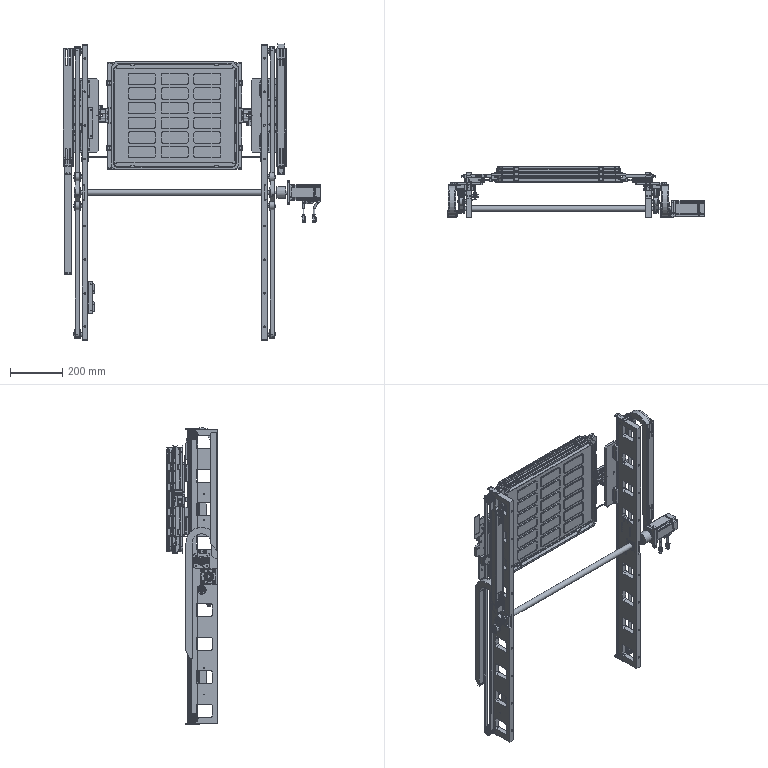Part | NX | 124 solids | 8566 faces | volume 7833772 mm3 | plane 4542 | cylinder 3272 | spline 462 | cone 274 | torus 16 | commonest cylinder face diameters 10 x348 0.8 x250 1.2 x248 13 x220 3 x210 4 x172